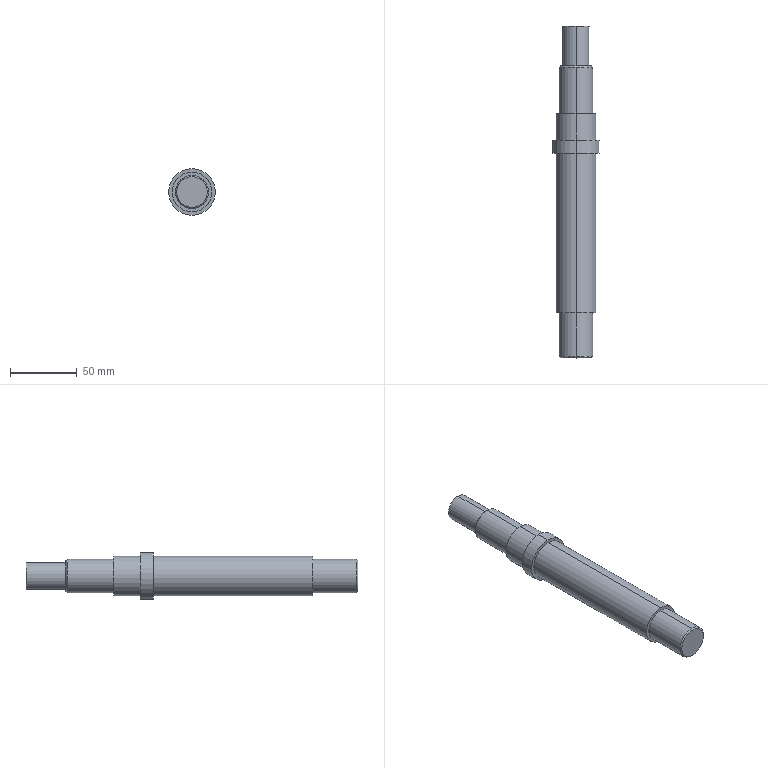Part | STEP file | 012-6-07-05 | 1 solid | 23 faces | box 35 x 249.4 x 35 mm | volume 151867 mm3 | cylinder 12 | plane 7 | cone 4 | commonest cylinder face diameters 25 x4 30 x4 20 x2 35 x2
STEP:
#1=CARTESIAN_POINT('',(0.,0.,0.));
#2=DIRECTION('',(0.,0.,1.));
#3=DIRECTION('',(1.,0.,0.));
#4=AXIS2_PLACEMENT_3D('',#1,#2,#3);
#5=CARTESIAN_POINT('',(0.,219.4,11.5));
#6=VERTEX_POINT('',#5);
#7=CARTESIAN_POINT('',(0.,219.4,-11.5));
#8=VERTEX_POINT('',#7);
#9=CARTESIAN_POINT('',(0.,219.4,0.));
#10=DIRECTION('',(0.,1.,0.));
#11=DIRECTION('',(0.,0.,1.));
#12=AXIS2_PLACEMENT_3D('',#9,#10,#11);
#13=CIRCLE('',#12,11.5);
#14=CARTESIAN_POINT('',(0.,218.4,0.));
#15=DIRECTION('',(0.,-1.,0.));
#16=DIRECTION('',(0.,0.,-1.));
#17=AXIS2_PLACEMENT_3D('',#14,#15,#16);
#18=CONICAL_SURFACE('',#17,12.5,0.7854);
#19=CARTESIAN_POINT('',(3.142,-1.));
#20=DIRECTION('',(-1.,0.));
#21=VECTOR('',#20,1.);
#22=LINE('',#19,#21);
#23=(GEOMETRIC_REPRESENTATION_CONTEXT(2)PARAMETRIC_REPRESENTATION_CONTEXT()REPRESENTATION_CONTEXT('',''));
#24=DEFINITIONAL_REPRESENTATION('',(#22),#23);
#25=PCURVE('',#18,#24);
#26=CARTESIAN_POINT('',(12.5,219.4,0.));
#27=DIRECTION('',(0.,1.,0.));
#28=DIRECTION('',(0.,0.,1.));
#29=AXIS2_PLACEMENT_3D('',#26,#27,#28);
#30=PLANE('',#29);
#31=CARTESIAN_POINT('',(0.,-12.5));
#32=DIRECTION('',(1.,0.));
#33=AXIS2_PLACEMENT_2D('',#31,#32);
#34=CIRCLE('',#33,11.5);
#35=(GEOMETRIC_REPRESENTATION_CONTEXT(2)PARAMETRIC_REPRESENTATION_CONTEXT()REPRESENTATION_CONTEXT('',''));
#36=DEFINITIONAL_REPRESENTATION('',(#34),#35);
#37=PCURVE('',#30,#36);
#38=SURFACE_CURVE('',#13,(#25,#37),.PCURVE_S1.);
#39=EDGE_CURVE('',#6,#8,#38,.T.);
#40=ORIENTED_EDGE('',*,*,#39,.F.);
#41=CARTESIAN_POINT('',(0.,218.4,12.5));
#42=VERTEX_POINT('',#41);
#43=CARTESIAN_POINT('',(0.,218.4,12.5));
#44=DIRECTION('',(0.,-0.7071,0.7071));
#45=VECTOR('',#44,1.);
#46=LINE('',#43,#45);
#47=CARTESIAN_POINT('',(3.142,0.));
#48=DIRECTION('',(0.,1.));
#49=VECTOR('',#48,1.);
#50=LINE('',#47,#49);
#51=(GEOMETRIC_REPRESENTATION_CONTEXT(2)PARAMETRIC_REPRESENTATION_CONTEXT()REPRESENTATION_CONTEXT('',''));
#52=DEFINITIONAL_REPRESENTATION('',(#50),#51);
#53=PCURVE('',#18,#52);
#54=CARTESIAN_POINT('',(0.,218.4,0.));
#55=DIRECTION('',(0.,-1.,0.));
#56=DIRECTION('',(0.,0.,-1.));
#57=AXIS2_PLACEMENT_3D('',#54,#55,#56);
#58=CONICAL_SURFACE('',#57,12.5,0.7854);
#59=CARTESIAN_POINT('',(3.142,0.));
#60=DIRECTION('',(0.,1.));
#61=VECTOR('',#60,1.);
#62=LINE('',#59,#61);
#63=(GEOMETRIC_REPRESENTATION_CONTEXT(2)PARAMETRIC_REPRESENTATION_CONTEXT()REPRESENTATION_CONTEXT('',''));
#64=DEFINITIONAL_REPRESENTATION('',(#62),#63);
#65=PCURVE('',#58,#64);
#66=SURFACE_CURVE('',#46,(#53,#65),.PCURVE_S1.);
#67=EDGE_CURVE('',#6,#42,#66,.T.);
#68=ORIENTED_EDGE('',*,*,#67,.T.);
#69=CARTESIAN_POINT('',(0.,218.4,-12.5));
#70=VERTEX_POINT('',#69);
#71=CARTESIAN_POINT('',(0.,218.4,0.));
#72=DIRECTION('',(0.,-1.,0.));
#73=DIRECTION('',(0.,0.,1.));
#74=AXIS2_PLACEMENT_3D('',#71,#72,#73);
#75=CIRCLE('',#74,12.5);
#76=CARTESIAN_POINT('',(-3.142,0.));
#77=DIRECTION('',(1.,0.));
#78=VECTOR('',#77,1.);
#79=LINE('',#76,#78);
#80=(GEOMETRIC_REPRESENTATION_CONTEXT(2)PARAMETRIC_REPRESENTATION_CONTEXT()REPRESENTATION_CONTEXT('',''));
#81=DEFINITIONAL_REPRESENTATION('',(#79),#80);
#82=PCURVE('',#18,#81);
#83=CARTESIAN_POINT('',(0.,0.,0.));
#84=DIRECTION('',(0.,-1.,0.));
#85=DIRECTION('',(0.,0.,-1.));
#86=AXIS2_PLACEMENT_3D('',#83,#84,#85);
#87=CYLINDRICAL_SURFACE('',#86,12.5);
#88=CARTESIAN_POINT('',(-3.142,-218.4));
#89=DIRECTION('',(1.,0.));
#90=VECTOR('',#89,1.);
#91=LINE('',#88,#90);
#92=(GEOMETRIC_REPRESENTATION_CONTEXT(2)PARAMETRIC_REPRESENTATION_CONTEXT()REPRESENTATION_CONTEXT('',''));
#93=DEFINITIONAL_REPRESENTATION('',(#91),#92);
#94=PCURVE('',#87,#93);
#95=SURFACE_CURVE('',#75,(#82,#94),.PCURVE_S1.);
#96=EDGE_CURVE('',#70,#42,#95,.T.);
#97=ORIENTED_EDGE('',*,*,#96,.F.);
#98=CARTESIAN_POINT('',(0.,218.4,-12.5));
#99=DIRECTION('',(0.,-0.7071,-0.7071));
#100=VECTOR('',#99,1.);
#101=LINE('',#98,#100);
#102=CARTESIAN_POINT('',(0.,0.));
#103=DIRECTION('',(0.,1.));
#104=VECTOR('',#103,1.);
#105=LINE('',#102,#104);
#106=(GEOMETRIC_REPRESENTATION_CONTEXT(2)PARAMETRIC_REPRESENTATION_CONTEXT()REPRESENTATION_CONTEXT('',''));
#107=DEFINITIONAL_REPRESENTATION('',(#105),#106);
#108=PCURVE('',#18,#107);
#109=CARTESIAN_POINT('',(6.283,0.));
#110=DIRECTION('',(0.,1.));
#111=VECTOR('',#110,1.);
#112=LINE('',#109,#111);
#113=(GEOMETRIC_REPRESENTATION_CONTEXT(2)PARAMETRIC_REPRESENTATION_CONTEXT()REPRESENTATION_CONTEXT('',''));
#114=DEFINITIONAL_REPRESENTATION('',(#112),#113);
#115=PCURVE('',#58,#114);
#116=SURFACE_CURVE('',#101,(#108,#115),.PCURVE_S1.);
#117=EDGE_CURVE('',#8,#70,#116,.T.);
#118=ORIENTED_EDGE('',*,*,#117,.F.);
#119=EDGE_LOOP('',(#40,#68,#97,#118));
#120=FACE_BOUND('',#119,.T.);
#121=ADVANCED_FACE('',(#120),#18,.T.);
#122=CARTESIAN_POINT('',(0.,0.,-11.5));
#123=VERTEX_POINT('',#122);
#124=CARTESIAN_POINT('',(0.,0.,11.5));
#125=VERTEX_POINT('',#124);
#126=CARTESIAN_POINT('',(0.,0.,0.));
#127=DIRECTION('',(0.,-1.,0.));
#128=DIRECTION('',(0.,0.,-1.));
#129=AXIS2_PLACEMENT_3D('',#126,#127,#128);
#130=CIRCLE('',#129,11.5);
#131=CARTESIAN_POINT('',(0.,0.,0.));
#132=DIRECTION('',(0.,1.,0.));
#133=DIRECTION('',(0.,0.,1.));
#134=AXIS2_PLACEMENT_3D('',#131,#132,#133);
#135=CONICAL_SURFACE('',#134,11.5,0.7854);
#136=CARTESIAN_POINT('',(3.142,0.));
#137=DIRECTION('',(-1.,0.));
#138=VECTOR('',#137,1.);
#139=LINE('',#136,#138);
#140=(GEOMETRIC_REPRESENTATION_CONTEXT(2)PARAMETRIC_REPRESENTATION_CONTEXT()REPRESENTATION_CONTEXT('',''));
#141=DEFINITIONAL_REPRESENTATION('',(#139),#140);
#142=PCURVE('',#135,#141);
#143=CARTESIAN_POINT('',(0.,0.,0.));
#144=DIRECTION('',(0.,-1.,0.));
#145=DIRECTION('',(0.,0.,-1.));
#146=AXIS2_PLACEMENT_3D('',#143,#144,#145);
#147=PLANE('',#146);
#148=CARTESIAN_POINT('',(0.,0.));
#149=DIRECTION('',(1.,0.));
#150=AXIS2_PLACEMENT_2D('',#148,#149);
#151=CIRCLE('',#150,11.5);
#152=(GEOMETRIC_REPRESENTATION_CONTEXT(2)PARAMETRIC_REPRESENTATION_CONTEXT()REPRESENTATION_CONTEXT('',''));
#153=DEFINITIONAL_REPRESENTATION('',(#151),#152);
#154=PCURVE('',#147,#153);
#155=SURFACE_CURVE('',#130,(#142,#154),.PCURVE_S1.);
#156=EDGE_CURVE('',#123,#125,#155,.T.);
#157=ORIENTED_EDGE('',*,*,#156,.F.);
#158=CARTESIAN_POINT('',(0.,1.,-12.5));
#159=VERTEX_POINT('',#158);
#160=CARTESIAN_POINT('',(0.,0.,-11.5));
#161=DIRECTION('',(0.,0.7071,-0.7071));
#162=VECTOR('',#161,1.);
#163=LINE('',#160,#162);
#164=CARTESIAN_POINT('',(3.142,0.));
#165=DIRECTION('',(0.,1.));
#166=VECTOR('',#165,1.);
#167=LINE('',#164,#166);
#168=(GEOMETRIC_REPRESENTATION_CONTEXT(2)PARAMETRIC_REPRESENTATION_CONTEXT()REPRESENTATION_CONTEXT('',''));
#169=DEFINITIONAL_REPRESENTATION('',(#167),#168);
#170=PCURVE('',#135,#169);
#171=CARTESIAN_POINT('',(0.,0.,0.));
#172=DIRECTION('',(0.,1.,0.));
#173=DIRECTION('',(0.,0.,1.));
#174=AXIS2_PLACEMENT_3D('',#171,#172,#173);
#175=CONICAL_SURFACE('',#174,11.5,0.7854);
#176=CARTESIAN_POINT('',(3.142,0.));
#177=DIRECTION('',(0.,1.));
#178=VECTOR('',#177,1.);
#179=LINE('',#176,#178);
#180=(GEOMETRIC_REPRESENTATION_CONTEXT(2)PARAMETRIC_REPRESENTATION_CONTEXT()REPRESENTATION_CONTEXT('',''));
#181=DEFINITIONAL_REPRESENTATION('',(#179),#180);
#182=PCURVE('',#175,#181);
#183=SURFACE_CURVE('',#163,(#170,#182),.PCURVE_S1.);
#184=EDGE_CURVE('',#123,#159,#183,.T.);
#185=ORIENTED_EDGE('',*,*,#184,.T.);
#186=CARTESIAN_POINT('',(0.,1.,12.5));
#187=VERTEX_POINT('',#186);
#188=CARTESIAN_POINT('',(0.,1.,0.));
#189=DIRECTION('',(0.,1.,0.));
#190=DIRECTION('',(0.,0.,-1.));
#191=AXIS2_PLACEMENT_3D('',#188,#189,#190);
#192=CIRCLE('',#191,12.5);
#193=CARTESIAN_POINT('',(-3.142,1.));
#194=DIRECTION('',(1.,0.));
#195=VECTOR('',#194,1.);
#196=LINE('',#193,#195);
#197=(GEOMETRIC_REPRESENTATION_CONTEXT(2)PARAMETRIC_REPRESENTATION_CONTEXT()REPRESENTATION_CONTEXT('',''));
#198=DEFINITIONAL_REPRESENTATION('',(#196),#197);
#199=PCURVE('',#135,#198);
#200=CARTESIAN_POINT('',(0.,0.,0.));
#201=DIRECTION('',(0.,-1.,0.));
#202=DIRECTION('',(0.,0.,-1.));
#203=AXIS2_PLACEMENT_3D('',#200,#201,#202);
#204=CYLINDRICAL_SURFACE('',#203,12.5);
#205=CARTESIAN_POINT('',(6.283,-1.));
#206=DIRECTION('',(-1.,0.));
#207=VECTOR('',#206,1.);
#208=LINE('',#205,#207);
#209=(GEOMETRIC_REPRESENTATION_CONTEXT(2)PARAMETRIC_REPRESENTATION_CONTEXT()REPRESENTATION_CONTEXT('',''));
#210=DEFINITIONAL_REPRESENTATION('',(#208),#209);
#211=PCURVE('',#204,#210);
#212=SURFACE_CURVE('',#192,(#199,#211),.PCURVE_S1.);
#213=EDGE_CURVE('',#187,#159,#212,.T.);
#214=ORIENTED_EDGE('',*,*,#213,.F.);
#215=CARTESIAN_POINT('',(0.,0.,11.5));
#216=DIRECTION('',(0.,0.7071,0.7071));
#217=VECTOR('',#216,1.);
#218=LINE('',#215,#217);
#219=CARTESIAN_POINT('',(0.,0.));
#220=DIRECTION('',(0.,1.));
#221=VECTOR('',#220,1.);
#222=LINE('',#219,#221);
#223=(GEOMETRIC_REPRESENTATION_CONTEXT(2)PARAMETRIC_REPRESENTATION_CONTEXT()REPRESENTATION_CONTEXT('',''));
#224=DEFINITIONAL_REPRESENTATION('',(#222),#223);
#225=PCURVE('',#135,#224);
#226=CARTESIAN_POINT('',(6.283,0.));
#227=DIRECTION('',(0.,1.));
#228=VECTOR('',#227,1.);
#229=LINE('',#226,#228);
#230=(GEOMETRIC_REPRESENTATION_CONTEXT(2)PARAMETRIC_REPRESENTATION_CONTEXT()REPRESENTATION_CONTEXT('',''));
#231=DEFINITIONAL_REPRESENTATION('',(#229),#230);
#232=PCURVE('',#175,#231);
#233=SURFACE_CURVE('',#218,(#225,#232),.PCURVE_S1.);
#234=EDGE_CURVE('',#125,#187,#233,.T.);
#235=ORIENTED_EDGE('',*,*,#234,.F.);
#236=EDGE_LOOP('',(#157,#185,#214,#235));
#237=FACE_BOUND('',#236,.T.);
#238=ADVANCED_FACE('',(#237),#135,.T.);
#239=CARTESIAN_POINT('',(0.,249.4,-10.));
#240=VERTEX_POINT('',#239);
#241=CARTESIAN_POINT('',(0.,249.4,10.));
#242=VERTEX_POINT('',#241);
#243=CARTESIAN_POINT('',(0.,249.4,0.));
#244=DIRECTION('',(0.,-1.,0.));
#245=DIRECTION('',(0.,0.,-1.));
#246=AXIS2_PLACEMENT_3D('',#243,#244,#245);
#247=CIRCLE('',#246,10.);
#248=CARTESIAN_POINT('',(0.,0.,0.));
#249=DIRECTION('',(0.,-1.,0.));
#250=DIRECTION('',(0.,0.,-1.));
#251=AXIS2_PLACEMENT_3D('',#248,#249,#250);
#252=CYLINDRICAL_SURFACE('',#251,10.);
#253=CARTESIAN_POINT('',(0.,-249.4));
#254=DIRECTION('',(1.,0.));
#255=VECTOR('',#254,1.);
#256=LINE('',#253,#255);
#257=(GEOMETRIC_REPRESENTATION_CONTEXT(2)PARAMETRIC_REPRESENTATION_CONTEXT()REPRESENTATION_CONTEXT('',''));
#258=DEFINITIONAL_REPRESENTATION('',(#256),#257);
#259=PCURVE('',#252,#258);
#260=CARTESIAN_POINT('',(0.,249.4,0.));
#261=DIRECTION('',(0.,1.,0.));
#262=DIRECTION('',(0.,0.,1.));
#263=AXIS2_PLACEMENT_3D('',#260,#261,#262);
#264=PLANE('',#263);
#265=CARTESIAN_POINT('',(-10.,0.));
#266=CARTESIAN_POINT('',(-10.,17.321));
#267=CARTESIAN_POINT('',(5.,8.66));
#268=CARTESIAN_POINT('',(20.,0.));
#269=CARTESIAN_POINT('',(5.,-8.66));
#270=CARTESIAN_POINT('',(-10.,-17.321));
#271=CARTESIAN_POINT('',(-10.,0.));
#272=(BOUNDED_CURVE()B_SPLINE_CURVE(2,(#265,#266,#267,#268,#269,#270,#271),.UNSPECIFIED.,.T.,.F.)B_SPLINE_CURVE_WITH_KNOTS((1,2,2,2,2,1),(-2.094,0.,2.094,4.189,6.283,8.378),.UNSPECIFIED.)CURVE()GEOMETRIC_REPRESENTATION_ITEM()RATIONAL_B_SPLINE_CURVE((1.,0.5,1.,0.5,1.,0.5,1.))REPRESENTATION_ITEM(''));
#273=(GEOMETRIC_REPRESENTATION_CONTEXT(2)PARAMETRIC_REPRESENTATION_CONTEXT()REPRESENTATION_CONTEXT('',''));
#274=DEFINITIONAL_REPRESENTATION('',(#272),#273);
#275=PCURVE('',#264,#274);
#276=SURFACE_CURVE('',#247,(#259,#275),.PCURVE_S1.);
#277=EDGE_CURVE('',#240,#242,#276,.T.);
#278=ORIENTED_EDGE('',*,*,#277,.T.);
#279=CARTESIAN_POINT('',(0.,219.4,10.));
#280=VERTEX_POINT('',#279);
#281=CARTESIAN_POINT('',(0.,0.,10.));
#282=DIRECTION('',(0.,-1.,0.));
#283=VECTOR('',#282,1.);
#284=LINE('',#281,#283);
#285=CARTESIAN_POINT('',(3.142,0.));
#286=DIRECTION('',(0.,1.));
#287=VECTOR('',#286,1.);
#288=LINE('',#285,#287);
#289=(GEOMETRIC_REPRESENTATION_CONTEXT(2)PARAMETRIC_REPRESENTATION_CONTEXT()REPRESENTATION_CONTEXT('',''));
#290=DEFINITIONAL_REPRESENTATION('',(#288),#289);
#291=PCURVE('',#252,#290);
#292=CARTESIAN_POINT('',(0.,0.,0.));
#293=DIRECTION('',(0.,-1.,0.));
#294=DIRECTION('',(0.,0.,-1.));
#295=AXIS2_PLACEMENT_3D('',#292,#293,#294);
#296=CYLINDRICAL_SURFACE('',#295,10.);
#297=CARTESIAN_POINT('',(3.142,0.));
#298=DIRECTION('',(0.,1.));
#299=VECTOR('',#298,1.);
#300=LINE('',#297,#299);
#301=(GEOMETRIC_REPRESENTATION_CONTEXT(2)PARAMETRIC_REPRESENTATION_CONTEXT()REPRESENTATION_CONTEXT('',''));
#302=DEFINITIONAL_REPRESENTATION('',(#300),#301);
#303=PCURVE('',#296,#302);
#304=SURFACE_CURVE('',#284,(#291,#303),.PCURVE_S1.);
#305=EDGE_CURVE('',#242,#280,#304,.T.);
#306=ORIENTED_EDGE('',*,*,#305,.T.);
#307=CARTESIAN_POINT('',(0.,219.4,-10.));
#308=VERTEX_POINT('',#307);
#309=CARTESIAN_POINT('',(0.,219.4,0.));
#310=DIRECTION('',(0.,-1.,0.));
#311=DIRECTION('',(0.,0.,-1.));
#312=AXIS2_PLACEMENT_3D('',#309,#310,#311);
#313=CIRCLE('',#312,10.);
#314=CARTESIAN_POINT('',(0.,-219.4));
#315=DIRECTION('',(1.,0.));
#316=VECTOR('',#315,1.);
#317=LINE('',#314,#316);
#318=(GEOMETRIC_REPRESENTATION_CONTEXT(2)PARAMETRIC_REPRESENTATION_CONTEXT()REPRESENTATION_CONTEXT('',''));
#319=DEFINITIONAL_REPRESENTATION('',(#317),#318);
#320=PCURVE('',#252,#319);
#321=CARTESIAN_POINT('',(-10.,-12.5));
#322=CARTESIAN_POINT('',(-10.,4.821));
#323=CARTESIAN_POINT('',(5.,-3.84));
#324=CARTESIAN_POINT('',(20.,-12.5));
#325=CARTESIAN_POINT('',(5.,-21.16));
#326=CARTESIAN_POINT('',(-10.,-29.821));
#327=CARTESIAN_POINT('',(-10.,-12.5));
#328=(BOUNDED_CURVE()B_SPLINE_CURVE(2,(#321,#322,#323,#324,#325,#326,#327),.UNSPECIFIED.,.T.,.F.)B_SPLINE_CURVE_WITH_KNOTS((1,2,2,2,2,1),(-2.094,0.,2.094,4.189,6.283,8.378),.UNSPECIFIED.)CURVE()GEOMETRIC_REPRESENTATION_ITEM()RATIONAL_B_SPLINE_CURVE((1.,0.5,1.,0.5,1.,0.5,1.))REPRESENTATION_ITEM(''));
#329=(GEOMETRIC_REPRESENTATION_CONTEXT(2)PARAMETRIC_REPRESENTATION_CONTEXT()REPRESENTATION_CONTEXT('',''));
#330=DEFINITIONAL_REPRESENTATION('',(#328),#329);
#331=PCURVE('',#30,#330);
#332=SURFACE_CURVE('',#313,(#320,#331),.PCURVE_S1.);
#333=EDGE_CURVE('',#308,#280,#332,.T.);
#334=ORIENTED_EDGE('',*,*,#333,.F.);
#335=CARTESIAN_POINT('',(0.,0.,-10.));
#336=DIRECTION('',(0.,-1.,0.));
#337=VECTOR('',#336,1.);
#338=LINE('',#335,#337);
#339=CARTESIAN_POINT('',(0.,0.));
#340=DIRECTION('',(0.,1.));
#341=VECTOR('',#340,1.);
#342=LINE('',#339,#341);
#343=(GEOMETRIC_REPRESENTATION_CONTEXT(2)PARAMETRIC_REPRESENTATION_CONTEXT()REPRESENTATION_CONTEXT('',''));
#344=DEFINITIONAL_REPRESENTATION('',(#342),#343);
#345=PCURVE('',#252,#344);
#346=CARTESIAN_POINT('',(6.283,0.));
#347=DIRECTION('',(0.,1.));
#348=VECTOR('',#347,1.);
#349=LINE('',#346,#348);
#350=(GEOMETRIC_REPRESENTATION_CONTEXT(2)PARAMETRIC_REPRESENTATION_CONTEXT()REPRESENTATION_CONTEXT('',''));
#351=DEFINITIONAL_REPRESENTATION('',(#349),#350);
#352=PCURVE('',#296,#351);
#353=SURFACE_CURVE('',#338,(#345,#352),.PCURVE_S1.);
#354=EDGE_CURVE('',#240,#308,#353,.T.);
#355=ORIENTED_EDGE('',*,*,#354,.F.);
#356=EDGE_LOOP('',(#278,#306,#334,#355));
#357=FACE_BOUND('',#356,.T.);
#358=ADVANCED_FACE('',(#357),#252,.T.);
#359=ORIENTED_EDGE('',*,*,#96,.T.);
#360=CARTESIAN_POINT('',(0.,183.4,12.5));
#361=VERTEX_POINT('',#360);
#362=CARTESIAN_POINT('',(0.,0.,12.5));
#363=DIRECTION('',(0.,-1.,0.));
#364=VECTOR('',#363,1.);
#365=LINE('',#362,#364);
#366=CARTESIAN_POINT('',(3.142,0.));
#367=DIRECTION('',(0.,1.));
#368=VECTOR('',#367,1.);
#369=LINE('',#366,#368);
#370=(GEOMETRIC_REPRESENTATION_CONTEXT(2)PARAMETRIC_REPRESENTATION_CONTEXT()REPRESENTATION_CONTEXT('',''));
#371=DEFINITIONAL_REPRESENTATION('',(#369),#370);
#372=PCURVE('',#87,#371);
#373=CARTESIAN_POINT('',(0.,0.,0.));
#374=DIRECTION('',(0.,-1.,0.));
#375=DIRECTION('',(0.,0.,-1.));
#376=AXIS2_PLACEMENT_3D('',#373,#374,#375);
#377=CYLINDRICAL_SURFACE('',#376,12.5);
#378=CARTESIAN_POINT('',(3.142,0.));
#379=DIRECTION('',(0.,1.));
#380=VECTOR('',#379,1.);
#381=LINE('',#378,#380);
#382=(GEOMETRIC_REPRESENTATION_CONTEXT(2)PARAMETRIC_REPRESENTATION_CONTEXT()REPRESENTATION_CONTEXT('',''));
#383=DEFINITIONAL_REPRESENTATION('',(#381),#382);
#384=PCURVE('',#377,#383);
#385=SURFACE_CURVE('',#365,(#372,#384),.PCURVE_S1.);
#386=EDGE_CURVE('',#42,#361,#385,.T.);
#387=ORIENTED_EDGE('',*,*,#386,.T.);
#388=CARTESIAN_POINT('',(0.,183.4,-12.5));
#389=VERTEX_POINT('',#388);
#390=CARTESIAN_POINT('',(0.,183.4,0.));
#391=DIRECTION('',(0.,-1.,0.));
#392=DIRECTION('',(0.,0.,-1.));
#393=AXIS2_PLACEMENT_3D('',#390,#391,#392);
#394=CIRCLE('',#393,12.5);
#395=CARTESIAN_POINT('',(0.,-183.4));
#396=DIRECTION('',(1.,0.));
#397=VECTOR('',#396,1.);
#398=LINE('',#395,#397);
#399=(GEOMETRIC_REPRESENTATION_CONTEXT(2)PARAMETRIC_REPRESENTATION_CONTEXT()REPRESENTATION_CONTEXT('',''));
#400=DEFINITIONAL_REPRESENTATION('',(#398),#399);
#401=PCURVE('',#87,#400);
#402=CARTESIAN_POINT('',(12.5,183.4,0.));
#403=DIRECTION('',(0.,1.,0.));
#404=DIRECTION('',(0.,0.,1.));
#405=AXIS2_PLACEMENT_3D('',#402,#403,#404);
#406=PLANE('',#405);
#407=CARTESIAN_POINT('',(-12.5,-12.5));
#408=CARTESIAN_POINT('',(-12.5,9.151));
#409=CARTESIAN_POINT('',(6.25,-1.675));
#410=CARTESIAN_POINT('',(25.,-12.5));
#411=CARTESIAN_POINT('',(6.25,-23.325));
#412=CARTESIAN_POINT('',(-12.5,-34.151));
#413=CARTESIAN_POINT('',(-12.5,-12.5));
#414=(BOUNDED_CURVE()B_SPLINE_CURVE(2,(#407,#408,#409,#410,#411,#412,#413),.UNSPECIFIED.,.T.,.F.)B_SPLINE_CURVE_WITH_KNOTS((1,2,2,2,2,1),(-2.094,0.,2.094,4.189,6.283,8.378),.UNSPECIFIED.)CURVE()GEOMETRIC_REPRESENTATION_ITEM()RATIONAL_B_SPLINE_CURVE((1.,0.5,1.,0.5,1.,0.5,1.))REPRESENTATION_ITEM(''));
#415=(GEOMETRIC_REPRESENTATION_CONTEXT(2)PARAMETRIC_REPRESENTATION_CONTEXT()REPRESENTATION_CONTEXT('',''));
#416=DEFINITIONAL_REPRESENTATION('',(#414),#415);
#417=PCURVE('',#406,#416);
#418=SURFACE_CURVE('',#394,(#401,#417),.PCURVE_S1.);
#419=EDGE_CURVE('',#389,#361,#418,.T.);
#420=ORIENTED_EDGE('',*,*,#419,.F.);
#421=CARTESIAN_POINT('',(0.,0.,-12.5));
#422=DIRECTION('',(0.,-1.,0.));
#423=VECTOR('',#422,1.);
#424=LINE('',#421,#423);
#425=CARTESIAN_POINT('',(0.,0.));
#426=DIRECTION('',(0.,1.));
#427=VECTOR('',#426,1.);
#428=LINE('',#425,#427);
#429=(GEOMETRIC_REPRESENTATION_CONTEXT(2)PARAMETRIC_REPRESENTATION_CONTEXT()REPRESENTATION_CONTEXT('',''));
#430=DEFINITIONAL_REPRESENTATION('',(#428),#429);
#431=PCURVE('',#87,#430);
#432=CARTESIAN_POINT('',(6.283,0.));
#433=DIRECTION('',(0.,1.));
#434=VECTOR('',#433,1.);
#435=LINE('',#432,#434);
#436=(GEOMETRIC_REPRESENTATION_CONTEXT(2)PARAMETRIC_REPRESENTATION_CONTEXT()REPRESENTATION_CONTEXT('',''));
#437=DEFINITIONAL_REPRESENTATION('',(#435),#436);
#438=PCURVE('',#377,#437);
#439=SURFACE_CURVE('',#424,(#431,#438),.PCURVE_S1.);
#440=EDGE_CURVE('',#70,#389,#439,.T.);
#441=ORIENTED_EDGE('',*,*,#440,.F.);
#442=EDGE_LOOP('',(#359,#387,#420,#441));
#443=FACE_BOUND('',#442,.T.);
#444=ADVANCED_FACE('',(#443),#87,.T.);
#445=CARTESIAN_POINT('',(0.,183.4,-15.));
#446=VERTEX_POINT('',#445);
#447=CARTESIAN_POINT('',(0.,183.4,15.));
#448=VERTEX_POINT('',#447);
#449=CARTESIAN_POINT('',(0.,183.4,0.));
#450=DIRECTION('',(0.,-1.,0.));
#451=DIRECTION('',(0.,0.,-1.));
#452=AXIS2_PLACEMENT_3D('',#449,#450,#451);
#453=CIRCLE('',#452,15.);
#454=CARTESIAN_POINT('',(0.,0.,0.));
#455=DIRECTION('',(0.,-1.,0.));
#456=DIRECTION('',(0.,0.,-1.));
#457=AXIS2_PLACEMENT_3D('',#454,#455,#456);
#458=CYLINDRICAL_SURFACE('',#457,15.);
#459=CARTESIAN_POINT('',(0.,-183.4));
#460=DIRECTION('',(1.,0.));
#461=VECTOR('',#460,1.);
#462=LINE('',#459,#461);
#463=(GEOMETRIC_REPRESENTATION_CONTEXT(2)PARAMETRIC_REPRESENTATION_CONTEXT()REPRESENTATION_CONTEXT('',''));
#464=DEFINITIONAL_REPRESENTATION('',(#462),#463);
#465=PCURVE('',#458,#464);
#466=CARTESIAN_POINT('',(-15.,-12.5));
#467=CARTESIAN_POINT('',(-15.,13.481));
#468=CARTESIAN_POINT('',(7.5,0.4904));
#469=CARTESIAN_POINT('',(30.,-12.5));
#470=CARTESIAN_POINT('',(7.5,-25.49));
#471=CARTESIAN_POINT('',(-15.,-38.481));
#472=CARTESIAN_POINT('',(-15.,-12.5));
#473=(BOUNDED_CURVE()B_SPLINE_CURVE(2,(#466,#467,#468,#469,#470,#471,#472),.UNSPECIFIED.,.T.,.F.)B_SPLINE_CURVE_WITH_KNOTS((1,2,2,2,2,1),(-2.094,0.,2.094,4.189,6.283,8.378),.UNSPECIFIED.)CURVE()GEOMETRIC_REPRESENTATION_ITEM()RATIONAL_B_SPLINE_CURVE((1.,0.5,1.,0.5,1.,0.5,1.))REPRESENTATION_ITEM(''));
#474=(GEOMETRIC_REPRESENTATION_CONTEXT(2)PARAMETRIC_REPRESENTATION_CONTEXT()REPRESENTATION_CONTEXT('',''));
#475=DEFINITIONAL_REPRESENTATION('',(#473),#474);
#476=PCURVE('',#406,#475);
#477=SURFACE_CURVE('',#453,(#465,#476),.PCURVE_S1.);
#478=EDGE_CURVE('',#446,#448,#477,.T.);
#479=ORIENTED_EDGE('',*,*,#478,.T.);
#480=CARTESIAN_POINT('',(0.,163.7,15.));
#481=VERTEX_POINT('',#480);
#482=CARTESIAN_POINT('',(0.,0.,15.));
#483=DIRECTION('',(0.,-1.,0.));
#484=VECTOR('',#483,1.);
#485=LINE('',#482,#484);
#486=CARTESIAN_POINT('',(3.142,0.));
#487=DIRECTION('',(0.,1.));
#488=VECTOR('',#487,1.);
#489=LINE('',#486,#488);
#490=(GEOMETRIC_REPRESENTATION_CONTEXT(2)PARAMETRIC_REPRESENTATION_CONTEXT()REPRESENTATION_CONTEXT('',''));
#491=DEFINITIONAL_REPRESENTATION('',(#489),#490);
#492=PCURVE('',#458,#491);
#493=CARTESIAN_POINT('',(0.,0.,0.));
#494=DIRECTION('',(0.,-1.,0.));
#495=DIRECTION('',(0.,0.,-1.));
#496=AXIS2_PLACEMENT_3D('',#493,#494,#495);
#497=CYLINDRICAL_SURFACE('',#496,15.);
#498=CARTESIAN_POINT('',(3.142,0.));
#499=DIRECTION('',(0.,1.));
#500=VECTOR('',#499,1.);
#501=LINE('',#498,#500);
#502=(GEOMETRIC_REPRESENTATION_CONTEXT(2)PARAMETRIC_REPRESENTATION_CONTEXT()REPRESENTATION_CONTEXT('',''));
#503=DEFINITIONAL_REPRESENTATION('',(#501),#502);
#504=PCURVE('',#497,#503);
#505=SURFACE_CURVE('',#485,(#492,#504),.PCURVE_S1.);
#506=EDGE_CURVE('',#448,#481,#505,.T.);
#507=ORIENTED_EDGE('',*,*,#506,.T.);
#508=CARTESIAN_POINT('',(0.,163.7,-15.));
#509=VERTEX_POINT('',#508);
#510=CARTESIAN_POINT('',(0.,163.7,0.));
#511=DIRECTION('',(0.,-1.,0.));
#512=DIRECTION('',(0.,0.,-1.));
#513=AXIS2_PLACEMENT_3D('',#510,#511,#512);
#514=CIRCLE('',#513,15.);
#515=CARTESIAN_POINT('',(0.,-163.7));
#516=DIRECTION('',(1.,0.));
#517=VECTOR('',#516,1.);
#518=LINE('',#515,#517);
#519=(GEOMETRIC_REPRESENTATION_CONTEXT(2)PARAMETRIC_REPRESENTATION_CONTEXT()REPRESENTATION_CONTEXT('',''));
#520=DEFINITIONAL_REPRESENTATION('',(#518),#519);
#521=PCURVE('',#458,#520);
#522=CARTESIAN_POINT('',(15.,163.7,0.));
#523=DIRECTION('',(0.,1.,0.));
#524=DIRECTION('',(0.,0.,1.));
#525=AXIS2_PLACEMENT_3D('',#522,#523,#524);
#526=PLANE('',#525);
#527=CARTESIAN_POINT('',(-15.,-15.));
#528=CARTESIAN_POINT('',(-15.,10.981));
#529=CARTESIAN_POINT('',(7.5,-2.01));
#530=CARTESIAN_POINT('',(30.,-15.));
#531=CARTESIAN_POINT('',(7.5,-27.99));
#532=CARTESIAN_POINT('',(-15.,-40.981));
#533=CARTESIAN_POINT('',(-15.,-15.));
#534=(BOUNDED_CURVE()B_SPLINE_CURVE(2,(#527,#528,#529,#530,#531,#532,#533),.UNSPECIFIED.,.T.,.F.)B_SPLINE_CURVE_WITH_KNOTS((1,2,2,2,2,1),(-2.094,0.,2.094,4.189,6.283,8.378),.UNSPECIFIED.)CURVE()GEOMETRIC_REPRESENTATION_ITEM()RATIONAL_B_SPLINE_CURVE((1.,0.5,1.,0.5,1.,0.5,1.))REPRESENTATION_ITEM(''));
#535=(GEOMETRIC_REPRESENTATION_CONTEXT(2)PARAMETRIC_REPRESENTATION_CONTEXT()REPRESENTATION_CONTEXT('',''));
#536=DEFINITIONAL_REPRESENTATION('',(#534),#535);
#537=PCURVE('',#526,#536);
#538=SURFACE_CURVE('',#514,(#521,#537),.PCURVE_S1.);
#539=EDGE_CURVE('',#509,#481,#538,.T.);
#540=ORIENTED_EDGE('',*,*,#539,.F.);
#541=CARTESIAN_POINT('',(0.,0.,-15.));
#542=DIRECTION('',(0.,-1.,0.));
#543=VECTOR('',#542,1.);
#544=LINE('',#541,#543);
#545=CARTESIAN_POINT('',(0.,0.));
#546=DIRECTION('',(0.,1.));
#547=VECTOR('',#546,1.);
#548=LINE('',#545,#547);
#549=(GEOMETRIC_REPRESENTATION_CONTEXT(2)PARAMETRIC_REPRESENTATION_CONTEXT()REPRESENTATION_CONTEXT('',''));
#550=DEFINITIONAL_REPRESENTATION('',(#548),#549);
#551=PCURVE('',#458,#550);
#552=CARTESIAN_POINT('',(6.283,0.));
#553=DIRECTION('',(0.,1.));
#554=VECTOR('',#553,1.);
#555=LINE('',#552,#554);
#556=(GEOMETRIC_REPRESENTATION_CONTEXT(2)PARAMETRIC_REPRESENTATION_CONTEXT()REPRESENTATION_CONTEXT('',''));
#557=DEFINITIONAL_REPRESENTATION('',(#555),#556);
#558=PCURVE('',#497,#557);
#559=SURFACE_CURVE('',#544,(#551,#558),.PCURVE_S1.);
#560=EDGE_CURVE('',#446,#509,#559,.T.);
#561=ORIENTED_EDGE('',*,*,#560,.F.);
#562=EDGE_LOOP('',(#479,#507,#540,#561));
#563=FACE_BOUND('',#562,.T.);
#564=ADVANCED_FACE('',(#563),#458,.T.);
#565=CARTESIAN_POINT('',(0.,163.7,-17.5));
#566=VERTEX_POINT('',#565);
#567=CARTESIAN_POINT('',(0.,163.7,17.5));
#568=VERTEX_POINT('',#567);
#569=CARTESIAN_POINT('',(0.,163.7,0.));
#570=DIRECTION('',(0.,-1.,0.));
#571=DIRECTION('',(0.,0.,-1.));
#572=AXIS2_PLACEMENT_3D('',#569,#570,#571);
#573=CIRCLE('',#572,17.5);
#574=CARTESIAN_POINT('',(0.,0.,0.));
#575=DIRECTION('',(0.,-1.,0.));
#576=DIRECTION('',(0.,0.,-1.));
#577=AXIS2_PLACEMENT_3D('',#574,#575,#576);
#578=CYLINDRICAL_SURFACE('',#577,17.5);
#579=CARTESIAN_POINT('',(0.,-163.7));
#580=DIRECTION('',(1.,0.));
#581=VECTOR('',#580,1.);
#582=LINE('',#579,#581);
#583=(GEOMETRIC_REPRESENTATION_CONTEXT(2)PARAMETRIC_REPRESENTATION_CONTEXT()REPRESENTATION_CONTEXT('',''));
#584=DEFINITIONAL_REPRESENTATION('',(#582),#583);
#585=PCURVE('',#578,#584);
#586=CARTESIAN_POINT('',(-17.5,-15.));
#587=CARTESIAN_POINT('',(-17.5,15.311));
#588=CARTESIAN_POINT('',(8.75,0.1554));
#589=CARTESIAN_POINT('',(35.,-15.));
#590=CARTESIAN_POINT('',(8.75,-30.155));
#591=CARTESIAN_POINT('',(-17.5,-45.311));
#592=CARTESIAN_POINT('',(-17.5,-15.));
#593=(BOUNDED_CURVE()B_SPLINE_CURVE(2,(#586,#587,#588,#589,#590,#591,#592),.UNSPECIFIED.,.T.,.F.)B_SPLINE_CURVE_WITH_KNOTS((1,2,2,2,2,1),(-2.094,0.,2.094,4.189,6.283,8.378),.UNSPECIFIED.)CURVE()GEOMETRIC_REPRESENTATION_ITEM()RATIONAL_B_SPLINE_CURVE((1.,0.5,1.,0.5,1.,0.5,1.))REPRESENTATION_ITEM(''));
#594=(GEOMETRIC_REPRESENTATION_CONTEXT(2)PARAMETRIC_REPRESENTATION_CONTEXT()REPRESENTATION_CONTEXT('',''));
#595=DEFINITIONAL_REPRESENTATION('',(#593),#594);
#596=PCURVE('',#526,#595);
#597=SURFACE_CURVE('',#573,(#585,#596),.PCURVE_S1.);
#598=EDGE_CURVE('',#566,#568,#597,.T.);
#599=ORIENTED_EDGE('',*,*,#598,.T.);
#600=CARTESIAN_POINT('',(0.,153.7,17.5));
#601=VERTEX_POINT('',#600);
#602=CARTESIAN_POINT('',(0.,0.,17.5));
#603=DIRECTION('',(0.,-1.,0.));
#604=VECTOR('',#603,1.);
#605=LINE('',#602,#604);
#606=CARTESIAN_POINT('',(3.142,0.));
#607=DIRECTION('',(0.,1.));
#608=VECTOR('',#607,1.);
#609=LINE('',#606,#608);
#610=(GEOMETRIC_REPRESENTATION_CONTEXT(2)PARAMETRIC_REPRESENTATION_CONTEXT()REPRESENTATION_CONTEXT('',''));
#611=DEFINITIONAL_REPRESENTATION('',(#609),#610);
#612=PCURVE('',#578,#611);
#613=CARTESIAN_POINT('',(0.,0.,0.));
#614=DIRECTION('',(0.,-1.,0.));
#615=DIRECTION('',(0.,0.,-1.));
#616=AXIS2_PLACEMENT_3D('',#613,#614,#615);
#617=CYLINDRICAL_SURFACE('',#616,17.5);
#618=CARTESIAN_POINT('',(3.142,0.));
#619=DIRECTION('',(0.,1.));
#620=VECTOR('',#619,1.);
#621=LINE('',#618,#620);
#622=(GEOMETRIC_REPRESENTATION_CONTEXT(2)PARAMETRIC_REPRESENTATION_CONTEXT()REPRESENTATION_CONTEXT('',''));
#623=DEFINITIONAL_REPRESENTATION('',(#621),#622);
#624=PCURVE('',#617,#623);
#625=SURFACE_CURVE('',#605,(#612,#624),.PCURVE_S1.);
#626=EDGE_CURVE('',#568,#601,#625,.T.);
#627=ORIENTED_EDGE('',*,*,#626,.T.);
#628=CARTESIAN_POINT('',(0.,153.7,-17.5));
#629=VERTEX_POINT('',#628);
#630=CARTESIAN_POINT('',(0.,153.7,0.));
#631=DIRECTION('',(0.,-1.,0.));
#632=DIRECTION('',(0.,0.,-1.));
#633=AXIS2_PLACEMENT_3D('',#630,#631,#632);
#634=CIRCLE('',#633,17.5);
#635=CARTESIAN_POINT('',(0.,-153.7));
#636=DIRECTION('',(1.,0.));
#637=VECTOR('',#636,1.);
#638=LINE('',#635,#637);
#639=(GEOMETRIC_REPRESENTATION_CONTEXT(2)PARAMETRIC_REPRESENTATION_CONTEXT()REPRESENTATION_CONTEXT('',''));
#640=DEFINITIONAL_REPRESENTATION('',(#638),#639);
#641=PCURVE('',#578,#640);
#642=CARTESIAN_POINT('',(17.5,153.7,0.));
#643=DIRECTION('',(0.,-1.,0.));
#644=DIRECTION('',(0.,0.,-1.));
#645=AXIS2_PLACEMENT_3D('',#642,#643,#644);
#646=PLANE('',#645);
#647=CARTESIAN_POINT('',(0.,-17.5));
#648=DIRECTION('',(1.,0.));
#649=AXIS2_PLACEMENT_2D('',#647,#648);
#650=CIRCLE('',#649,17.5);
#651=(GEOMETRIC_REPRESENTATION_CONTEXT(2)PARAMETRIC_REPRESENTATION_CONTEXT()REPRESENTATION_CONTEXT('',''));
#652=DEFINITIONAL_REPRESENTATION('',(#650),#651);
#653=PCURVE('',#646,#652);
#654=SURFACE_CURVE('',#634,(#641,#653),.PCURVE_S1.);
#655=EDGE_CURVE('',#629,#601,#654,.T.);
#656=ORIENTED_EDGE('',*,*,#655,.F.);
#657=CARTESIAN_POINT('',(0.,0.,-17.5));
#658=DIRECTION('',(0.,-1.,0.));
#659=VECTOR('',#658,1.);
#660=LINE('',#657,#659);
#661=CARTESIAN_POINT('',(0.,0.));
#662=DIRECTION('',(0.,1.));
#663=VECTOR('',#662,1.);
#664=LINE('',#661,#663);
#665=(GEOMETRIC_REPRESENTATION_CONTEXT(2)PARAMETRIC_REPRESENTATION_CONTEXT()REPRESENTATION_CONTEXT('',''));
#666=DEFINITIONAL_REPRESENTATION('',(#664),#665);
#667=PCURVE('',#578,#666);
#668=CARTESIAN_POINT('',(6.283,0.));
#669=DIRECTION('',(0.,1.));
#670=VECTOR('',#669,1.);
#671=LINE('',#668,#670);
#672=(GEOMETRIC_REPRESENTATION_CONTEXT(2)PARAMETRIC_REPRESENTATION_CONTEXT()REPRESENTATION_CONTEXT('',''));
#673=DEFINITIONAL_REPRESENTATION('',(#671),#672);
#674=PCURVE('',#617,#673);
#675=SURFACE_CURVE('',#660,(#667,#674),.PCURVE_S1.);
#676=EDGE_CURVE('',#566,#629,#675,.T.);
#677=ORIENTED_EDGE('',*,*,#676,.F.);
#678=EDGE_LOOP('',(#599,#627,#656,#677));
#679=FACE_BOUND('',#678,.T.);
#680=ADVANCED_FACE('',(#679),#578,.T.);
#681=CARTESIAN_POINT('',(0.,153.7,-15.));
#682=VERTEX_POINT('',#681);
#683=CARTESIAN_POINT('',(0.,153.7,15.));
#684=VERTEX_POINT('',#683);
#685=CARTESIAN_POINT('',(0.,153.7,0.));
#686=DIRECTION('',(0.,-1.,0.));
#687=DIRECTION('',(0.,0.,-1.));
#688=AXIS2_PLACEMENT_3D('',#685,#686,#687);
#689=CIRCLE('',#688,15.);
#690=CARTESIAN_POINT('',(0.,0.,0.));
#691=DIRECTION('',(0.,-1.,0.));
#692=DIRECTION('',(0.,0.,-1.));
#693=AXIS2_PLACEMENT_3D('',#690,#691,#692);
#694=CYLINDRICAL_SURFACE('',#693,15.);
#695=CARTESIAN_POINT('',(0.,-153.7));
#696=DIRECTION('',(1.,0.));
#697=VECTOR('',#696,1.);
#698=LINE('',#695,#697);
#699=(GEOMETRIC_REPRESENTATION_CONTEXT(2)PARAMETRIC_REPRESENTATION_CONTEXT()REPRESENTATION_CONTEXT('',''));
#700=DEFINITIONAL_REPRESENTATION('',(#698),#699);
#701=PCURVE('',#694,#700);
#702=CARTESIAN_POINT('',(0.,-17.5));
#703=DIRECTION('',(1.,0.));
#704=AXIS2_PLACEMENT_2D('',#702,#703);
#705=CIRCLE('',#704,15.);
#706=(GEOMETRIC_REPRESENTATION_CONTEXT(2)PARAMETRIC_REPRESENTATION_CONTEXT()REPRESENTATION_CONTEXT('',''));
#707=DEFINITIONAL_REPRESENTATION('',(#705),#706);
#708=PCURVE('',#646,#707);
#709=SURFACE_CURVE('',#689,(#701,#708),.PCURVE_S1.);
#710=EDGE_CURVE('',#682,#684,#709,.T.);
#711=ORIENTED_EDGE('',*,*,#710,.T.);
#712=CARTESIAN_POINT('',(0.,34.,15.));
#713=VERTEX_POINT('',#712);
#714=CARTESIAN_POINT('',(0.,0.,15.));
#715=DIRECTION('',(0.,-1.,0.));
#716=VECTOR('',#715,1.);
#717=LINE('',#714,#716);
#718=CARTESIAN_POINT('',(3.142,0.));
#719=DIRECTION('',(0.,1.));
#720=VECTOR('',#719,1.);
#721=LINE('',#718,#720);
#722=(GEOMETRIC_REPRESENTATION_CONTEXT(2)PARAMETRIC_REPRESENTATION_CONTEXT()REPRESENTATION_CONTEXT('',''));
#723=DEFINITIONAL_REPRESENTATION('',(#721),#722);
#724=PCURVE('',#694,#723);
#725=CARTESIAN_POINT('',(0.,0.,0.));
#726=DIRECTION('',(0.,-1.,0.));
#727=DIRECTION('',(0.,0.,-1.));
#728=AXIS2_PLACEMENT_3D('',#725,#726,#727);
#729=CYLINDRICAL_SURFACE('',#728,15.);
#730=CARTESIAN_POINT('',(3.142,0.));
#731=DIRECTION('',(0.,1.));
#732=VECTOR('',#731,1.);
#733=LINE('',#730,#732);
#734=(GEOMETRIC_REPRESENTATION_CONTEXT(2)PARAMETRIC_REPRESENTATION_CONTEXT()REPRESENTATION_CONTEXT('',''));
#735=DEFINITIONAL_REPRESENTATION('',(#733),#734);
#736=PCURVE('',#729,#735);
#737=SURFACE_CURVE('',#717,(#724,#736),.PCURVE_S1.);
#738=EDGE_CURVE('',#684,#713,#737,.T.);
#739=ORIENTED_EDGE('',*,*,#738,.T.);
#740=CARTESIAN_POINT('',(0.,34.,-15.));
#741=VERTEX_POINT('',#740);
#742=CARTESIAN_POINT('',(0.,34.,0.));
#743=DIRECTION('',(0.,-1.,0.));
#744=DIRECTION('',(0.,0.,-1.));
#745=AXIS2_PLACEMENT_3D('',#742,#743,#744);
#746=CIRCLE('',#745,15.);
#747=CARTESIAN_POINT('',(0.,-34.));
#748=DIRECTION('',(1.,0.));
#749=VECTOR('',#748,1.);
#750=LINE('',#747,#749);
#751=(GEOMETRIC_REPRESENTATION_CONTEXT(2)PARAMETRIC_REPRESENTATION_CONTEXT()REPRESENTATION_CONTEXT('',''));
#752=DEFINITIONAL_REPRESENTATION('',(#750),#751);
#753=PCURVE('',#694,#752);
#754=CARTESIAN_POINT('',(12.5,34.,0.));
#755=DIRECTION('',(0.,-1.,0.));
#756=DIRECTION('',(0.,0.,-1.));
#757=AXIS2_PLACEMENT_3D('',#754,#755,#756);
#758=PLANE('',#757);
#759=CARTESIAN_POINT('',(0.,-12.5));
#760=DIRECTION('',(1.,0.));
#761=AXIS2_PLACEMENT_2D('',#759,#760);
#762=CIRCLE('',#761,15.);
#763=(GEOMETRIC_REPRESENTATION_CONTEXT(2)PARAMETRIC_REPRESENTATION_CONTEXT()REPRESENTATION_CONTEXT('',''));
#764=DEFINITIONAL_REPRESENTATION('',(#762),#763);
#765=PCURVE('',#758,#764);
#766=SURFACE_CURVE('',#746,(#753,#765),.PCURVE_S1.);
#767=EDGE_CURVE('',#741,#713,#766,.T.);
#768=ORIENTED_EDGE('',*,*,#767,.F.);
#769=CARTESIAN_POINT('',(0.,0.,-15.));
#770=DIRECTION('',(0.,-1.,0.));
#771=VECTOR('',#770,1.);
#772=LINE('',#769,#771);
#773=CARTESIAN_POINT('',(0.,0.));
#774=DIRECTION('',(0.,1.));
#775=VECTOR('',#774,1.);
#776=LINE('',#773,#775);
#777=(GEOMETRIC_REPRESENTATION_CONTEXT(2)PARAMETRIC_REPRESENTATION_CONTEXT()REPRESENTATION_CONTEXT('',''));
#778=DEFINITIONAL_REPRESENTATION('',(#776),#777);
#779=PCURVE('',#694,#778);
#780=CARTESIAN_POINT('',(6.283,0.));
#781=DIRECTION('',(0.,1.));
#782=VECTOR('',#781,1.);
#783=LINE('',#780,#782);
#784=(GEOMETRIC_REPRESENTATION_CONTEXT(2)PARAMETRIC_REPRESENTATION_CONTEXT()REPRESENTATION_CONTEXT('',''));
#785=DEFINITIONAL_REPRESENTATION('',(#783),#784);
#786=PCURVE('',#729,#785);
#787=SURFACE_CURVE('',#772,(#779,#786),.PCURVE_S1.);
#788=EDGE_CURVE('',#682,#741,#787,.T.);
#789=ORIENTED_EDGE('',*,*,#788,.F.);
#790=EDGE_LOOP('',(#711,#739,#768,#789));
#791=FACE_BOUND('',#790,.T.);
#792=ADVANCED_FACE('',(#791),#694,.T.);
#793=CARTESIAN_POINT('',(0.,34.,-12.5));
#794=VERTEX_POINT('',#793);
#795=CARTESIAN_POINT('',(0.,34.,12.5));
#796=VERTEX_POINT('',#795);
#797=CARTESIAN_POINT('',(0.,34.,0.));
#798=DIRECTION('',(0.,-1.,0.));
#799=DIRECTION('',(0.,0.,-1.));
#800=AXIS2_PLACEMENT_3D('',#797,#798,#799);
#801=CIRCLE('',#800,12.5);
#802=CARTESIAN_POINT('',(0.,-34.));
#803=DIRECTION('',(1.,0.));
#804=VECTOR('',#803,1.);
#805=LINE('',#802,#804);
#806=(GEOMETRIC_REPRESENTATION_CONTEXT(2)PARAMETRIC_REPRESENTATION_CONTEXT()REPRESENTATION_CONTEXT('',''));
#807=DEFINITIONAL_REPRESENTATION('',(#805),#806);
#808=PCURVE('',#204,#807);
#809=CARTESIAN_POINT('',(0.,-12.5));
#810=DIRECTION('',(1.,0.));
#811=AXIS2_PLACEMENT_2D('',#809,#810);
#812=CIRCLE('',#811,12.5);
#813=(GEOMETRIC_REPRESENTATION_CONTEXT(2)PARAMETRIC_REPRESENTATION_CONTEXT()REPRESENTATION_CONTEXT('',''));
#814=DEFINITIONAL_REPRESENTATION('',(#812),#813);
#815=PCURVE('',#758,#814);
#816=SURFACE_CURVE('',#801,(#808,#815),.PCURVE_S1.);
#817=EDGE_CURVE('',#794,#796,#816,.T.);
#818=ORIENTED_EDGE('',*,*,#817,.T.);
#819=CARTESIAN_POINT('',(0.,0.,12.5));
#820=DIRECTION('',(0.,-1.,0.));
#821=VECTOR('',#820,1.);
#822=LINE('',#819,#821);
#823=CARTESIAN_POINT('',(3.142,0.));
#824=DIRECTION('',(0.,1.));
#825=VECTOR('',#824,1.);
#826=LINE('',#823,#825);
#827=(GEOMETRIC_REPRESENTATION_CONTEXT(2)PARAMETRIC_REPRESENTATION_CONTEXT()REPRESENTATION_CONTEXT('',''));
#828=DEFINITIONAL_REPRESENTATION('',(#826),#827);
#829=PCURVE('',#204,#828);
#830=CARTESIAN_POINT('',(0.,0.,0.));
#831=DIRECTION('',(0.,-1.,0.));
#832=DIRECTION('',(0.,0.,-1.));
#833=AXIS2_PLACEMENT_3D('',#830,#831,#832);
#834=CYLINDRICAL_SURFACE('',#833,12.5);
#835=CARTESIAN_POINT('',(3.142,0.));
#836=DIRECTION('',(0.,1.));
#837=VECTOR('',#836,1.);
#838=LINE('',#835,#837);
#839=(GEOMETRIC_REPRESENTATION_CONTEXT(2)PARAMETRIC_REPRESENTATION_CONTEXT()REPRESENTATION_CONTEXT('',''));
#840=DEFINITIONAL_REPRESENTATION('',(#838),#839);
#841=PCURVE('',#834,#840);
#842=SURFACE_CURVE('',#822,(#829,#841),.PCURVE_S1.);
#843=EDGE_CURVE('',#796,#187,#842,.T.);
#844=ORIENTED_EDGE('',*,*,#843,.T.);
#845=ORIENTED_EDGE('',*,*,#213,.T.);
#846=CARTESIAN_POINT('',(0.,0.,-12.5));
#847=DIRECTION('',(0.,-1.,0.));
#848=VECTOR('',#847,1.);
#849=LINE('',#846,#848);
#850=CARTESIAN_POINT('',(0.,0.));
#851=DIRECTION('',(0.,1.));
#852=VECTOR('',#851,1.);
#853=LINE('',#850,#852);
#854=(GEOMETRIC_REPRESENTATION_CONTEXT(2)PARAMETRIC_REPRESENTATION_CONTEXT()REPRESENTATION_CONTEXT('',''));
#855=DEFINITIONAL_REPRESENTATION('',(#853),#854);
#856=PCURVE('',#204,#855);
#857=CARTESIAN_POINT('',(6.283,0.));
#858=DIRECTION('',(0.,1.));
#859=VECTOR('',#858,1.);
#860=LINE('',#857,#859);
#861=(GEOMETRIC_REPRESENTATION_CONTEXT(2)PARAMETRIC_REPRESENTATION_CONTEXT()REPRESENTATION_CONTEXT('',''));
#862=DEFINITIONAL_REPRESENTATION('',(#860),#861);
#863=PCURVE('',#834,#862);
#864=SURFACE_CURVE('',#849,(#856,#863),.PCURVE_S1.);
#865=EDGE_CURVE('',#794,#159,#864,.T.);
#866=ORIENTED_EDGE('',*,*,#865,.F.);
#867=EDGE_LOOP('',(#818,#844,#845,#866));
#868=FACE_BOUND('',#867,.T.);
#869=ADVANCED_FACE('',(#868),#204,.T.);
#870=CARTESIAN_POINT('',(0.,0.,0.));
#871=DIRECTION('',(0.,-1.,0.));
#872=DIRECTION('',(0.,0.,-1.));
#873=AXIS2_PLACEMENT_3D('',#870,#871,#872);
#874=CIRCLE('',#873,11.5);
#875=CARTESIAN_POINT('',(0.,0.));
#876=DIRECTION('',(1.,0.));
#877=AXIS2_PLACEMENT_2D('',#875,#876);
#878=CIRCLE('',#877,11.5);
#879=(GEOMETRIC_REPRESENTATION_CONTEXT(2)PARAMETRIC_REPRESENTATION_CONTEXT()REPRESENTATION_CONTEXT('',''));
#880=DEFINITIONAL_REPRESENTATION('',(#878),#879);
#881=PCURVE('',#147,#880);
#882=CARTESIAN_POINT('',(9.425,0.));
#883=DIRECTION('',(-1.,0.));
#884=VECTOR('',#883,1.);
#885=LINE('',#882,#884);
#886=(GEOMETRIC_REPRESENTATION_CONTEXT(2)PARAMETRIC_REPRESENTATION_CONTEXT()REPRESENTATION_CONTEXT('',''));
#887=DEFINITIONAL_REPRESENTATION('',(#885),#886);
#888=PCURVE('',#175,#887);
#889=SURFACE_CURVE('',#874,(#881,#888),.PCURVE_S1.);
#890=EDGE_CURVE('',#125,#123,#889,.T.);
#891=ORIENTED_EDGE('',*,*,#890,.T.);
#892=ORIENTED_EDGE('',*,*,#156,.T.);
#893=EDGE_LOOP('',(#891,#892));
#894=FACE_BOUND('',#893,.T.);
#895=ADVANCED_FACE('',(#894),#147,.T.);
#896=ORIENTED_EDGE('',*,*,#843,.F.);
#897=CARTESIAN_POINT('',(0.,34.,0.));
#898=DIRECTION('',(0.,-1.,0.));
#899=DIRECTION('',(0.,0.,-1.));
#900=AXIS2_PLACEMENT_3D('',#897,#898,#899);
#901=CIRCLE('',#900,12.5);
#902=CARTESIAN_POINT('',(0.,-34.));
#903=DIRECTION('',(1.,0.));
#904=VECTOR('',#903,1.);
#905=LINE('',#902,#904);
#906=(GEOMETRIC_REPRESENTATION_CONTEXT(2)PARAMETRIC_REPRESENTATION_CONTEXT()REPRESENTATION_CONTEXT('',''));
#907=DEFINITIONAL_REPRESENTATION('',(#905),#906);
#908=PCURVE('',#834,#907);
#909=CARTESIAN_POINT('',(0.,-12.5));
#910=DIRECTION('',(1.,0.));
#911=AXIS2_PLACEMENT_2D('',#909,#910);
#912=CIRCLE('',#911,12.5);
#913=(GEOMETRIC_REPRESENTATION_CONTEXT(2)PARAMETRIC_REPRESENTATION_CONTEXT()REPRESENTATION_CONTEXT('',''));
#914=DEFINITIONAL_REPRESENTATION('',(#912),#913);
#915=PCURVE('',#758,#914);
#916=SURFACE_CURVE('',#901,(#908,#915),.PCURVE_S1.);
#917=EDGE_CURVE('',#796,#794,#916,.T.);
#918=ORIENTED_EDGE('',*,*,#917,.T.);
#919=ORIENTED_EDGE('',*,*,#865,.T.);
#920=CARTESIAN_POINT('',(0.,1.,0.));
#921=DIRECTION('',(0.,1.,0.));
#922=DIRECTION('',(0.,0.,-1.));
#923=AXIS2_PLACEMENT_3D('',#920,#921,#922);
#924=CIRCLE('',#923,12.5);
#925=CARTESIAN_POINT('',(6.283,-1.));
#926=DIRECTION('',(-1.,0.));
#927=VECTOR('',#926,1.);
#928=LINE('',#925,#927);
#929=(GEOMETRIC_REPRESENTATION_CONTEXT(2)PARAMETRIC_REPRESENTATION_CONTEXT()REPRESENTATION_CONTEXT('',''));
#930=DEFINITIONAL_REPRESENTATION('',(#928),#929);
#931=PCURVE('',#834,#930);
#932=CARTESIAN_POINT('',(3.142,1.));
#933=DIRECTION('',(1.,0.));
#934=VECTOR('',#933,1.);
#935=LINE('',#932,#934);
#936=(GEOMETRIC_REPRESENTATION_CONTEXT(2)PARAMETRIC_REPRESENTATION_CONTEXT()REPRESENTATION_CONTEXT('',''));
#937=DEFINITIONAL_REPRESENTATION('',(#935),#936);
#938=PCURVE('',#175,#937);
#939=SURFACE_CURVE('',#924,(#931,#938),.PCURVE_S1.);
#940=EDGE_CURVE('',#159,#187,#939,.T.);
#941=ORIENTED_EDGE('',*,*,#940,.T.);
#942=EDGE_LOOP('',(#896,#918,#919,#941));
#943=FACE_BOUND('',#942,.T.);
#944=ADVANCED_FACE('',(#943),#834,.T.);
#945=ORIENTED_EDGE('',*,*,#767,.T.);
#946=CARTESIAN_POINT('',(0.,34.,0.));
#947=DIRECTION('',(0.,-1.,0.));
#948=DIRECTION('',(0.,0.,-1.));
#949=AXIS2_PLACEMENT_3D('',#946,#947,#948);
#950=CIRCLE('',#949,15.);
#951=CARTESIAN_POINT('',(0.,-12.5));
#952=DIRECTION('',(1.,0.));
#953=AXIS2_PLACEMENT_2D('',#951,#952);
#954=CIRCLE('',#953,15.);
#955=(GEOMETRIC_REPRESENTATION_CONTEXT(2)PARAMETRIC_REPRESENTATION_CONTEXT()REPRESENTATION_CONTEXT('',''));
#956=DEFINITIONAL_REPRESENTATION('',(#954),#955);
#957=PCURVE('',#758,#956);
#958=CARTESIAN_POINT('',(0.,-34.));
#959=DIRECTION('',(1.,0.));
#960=VECTOR('',#959,1.);
#961=LINE('',#958,#960);
#962=(GEOMETRIC_REPRESENTATION_CONTEXT(2)PARAMETRIC_REPRESENTATION_CONTEXT()REPRESENTATION_CONTEXT('',''));
#963=DEFINITIONAL_REPRESENTATION('',(#961),#962);
#964=PCURVE('',#729,#963);
#965=SURFACE_CURVE('',#950,(#957,#964),.PCURVE_S1.);
#966=EDGE_CURVE('',#713,#741,#965,.T.);
#967=ORIENTED_EDGE('',*,*,#966,.T.);
#968=EDGE_LOOP('',(#945,#967));
#969=FACE_BOUND('',#968,.T.);
#970=ORIENTED_EDGE('',*,*,#817,.F.);
#971=ORIENTED_EDGE('',*,*,#917,.F.);
#972=EDGE_LOOP('',(#970,#971));
#973=FACE_BOUND('',#972,.T.);
#974=ADVANCED_FACE('',(#969,#973),#758,.T.);
#975=ORIENTED_EDGE('',*,*,#738,.F.);
#976=CARTESIAN_POINT('',(0.,153.7,0.));
#977=DIRECTION('',(0.,-1.,0.));
#978=DIRECTION('',(0.,0.,-1.));
#979=AXIS2_PLACEMENT_3D('',#976,#977,#978);
#980=CIRCLE('',#979,15.);
#981=CARTESIAN_POINT('',(0.,-153.7));
#982=DIRECTION('',(1.,0.));
#983=VECTOR('',#982,1.);
#984=LINE('',#981,#983);
#985=(GEOMETRIC_REPRESENTATION_CONTEXT(2)PARAMETRIC_REPRESENTATION_CONTEXT()REPRESENTATION_CONTEXT('',''));
#986=DEFINITIONAL_REPRESENTATION('',(#984),#985);
#987=PCURVE('',#729,#986);
#988=CARTESIAN_POINT('',(0.,-17.5));
#989=DIRECTION('',(1.,0.));
#990=AXIS2_PLACEMENT_2D('',#988,#989);
#991=CIRCLE('',#990,15.);
#992=(GEOMETRIC_REPRESENTATION_CONTEXT(2)PARAMETRIC_REPRESENTATION_CONTEXT()REPRESENTATION_CONTEXT('',''));
#993=DEFINITIONAL_REPRESENTATION('',(#991),#992);
#994=PCURVE('',#646,#993);
#995=SURFACE_CURVE('',#980,(#987,#994),.PCURVE_S1.);
#996=EDGE_CURVE('',#684,#682,#995,.T.);
#997=ORIENTED_EDGE('',*,*,#996,.T.);
#998=ORIENTED_EDGE('',*,*,#788,.T.);
#999=ORIENTED_EDGE('',*,*,#966,.F.);
#1000=EDGE_LOOP('',(#975,#997,#998,#999));
#1001=FACE_BOUND('',#1000,.T.);
#1002=ADVANCED_FACE('',(#1001),#729,.T.);
#1003=ORIENTED_EDGE('',*,*,#655,.T.);
#1004=CARTESIAN_POINT('',(0.,153.7,0.));
#1005=DIRECTION('',(0.,-1.,0.));
#1006=DIRECTION('',(0.,0.,-1.));
#1007=AXIS2_PLACEMENT_3D('',#1004,#1005,#1006);
#1008=CIRCLE('',#1007,17.5);
#1009=CARTESIAN_POINT('',(0.,-17.5));
#1010=DIRECTION('',(1.,0.));
#1011=AXIS2_PLACEMENT_2D('',#1009,#1010);
#1012=CIRCLE('',#1011,17.5);
#1013=(GEOMETRIC_REPRESENTATION_CONTEXT(2)PARAMETRIC_REPRESENTATION_CONTEXT()REPRESENTATION_CONTEXT('',''));
#1014=DEFINITIONAL_REPRESENTATION('',(#1012),#1013);
#1015=PCURVE('',#646,#1014);
#1016=CARTESIAN_POINT('',(0.,-153.7));
#1017=DIRECTION('',(1.,0.));
#1018=VECTOR('',#1017,1.);
#1019=LINE('',#1016,#1018);
#1020=(GEOMETRIC_REPRESENTATION_CONTEXT(2)PARAMETRIC_REPRESENTATION_CONTEXT()REPRESENTATION_CONTEXT('',''));
#1021=DEFINITIONAL_REPRESENTATION('',(#1019),#1020);
#1022=PCURVE('',#617,#1021);
#1023=SURFACE_CURVE('',#1008,(#1015,#1022),.PCURVE_S1.);
#1024=EDGE_CURVE('',#601,#629,#1023,.T.);
#1025=ORIENTED_EDGE('',*,*,#1024,.T.);
#1026=EDGE_LOOP('',(#1003,#1025));
#1027=FACE_BOUND('',#1026,.T.);
#1028=ORIENTED_EDGE('',*,*,#710,.F.);
#1029=ORIENTED_EDGE('',*,*,#996,.F.);
#1030=EDGE_LOOP('',(#1028,#1029));
#1031=FACE_BOUND('',#1030,.T.);
#1032=ADVANCED_FACE('',(#1027,#1031),#646,.T.);
#1033=ORIENTED_EDGE('',*,*,#626,.F.);
#1034=CARTESIAN_POINT('',(0.,163.7,0.));
#1035=DIRECTION('',(0.,-1.,0.));
#1036=DIRECTION('',(0.,0.,-1.));
#1037=AXIS2_PLACEMENT_3D('',#1034,#1035,#1036);
#1038=CIRCLE('',#1037,17.5);
#1039=CARTESIAN_POINT('',(0.,-163.7));
#1040=DIRECTION('',(1.,0.));
#1041=VECTOR('',#1040,1.);
#1042=LINE('',#1039,#1041);
#1043=(GEOMETRIC_REPRESENTATION_CONTEXT(2)PARAMETRIC_REPRESENTATION_CONTEXT()REPRESENTATION_CONTEXT('',''));
#1044=DEFINITIONAL_REPRESENTATION('',(#1042),#1043);
#1045=PCURVE('',#617,#1044);
#1046=CARTESIAN_POINT('',(-17.5,-15.));
#1047=CARTESIAN_POINT('',(-17.5,15.311));
#1048=CARTESIAN_POINT('',(8.75,0.1554));
#1049=CARTESIAN_POINT('',(35.,-15.));
#1050=CARTESIAN_POINT('',(8.75,-30.155));
#1051=CARTESIAN_POINT('',(-17.5,-45.311));
#1052=CARTESIAN_POINT('',(-17.5,-15.));
#1053=(BOUNDED_CURVE()B_SPLINE_CURVE(2,(#1046,#1047,#1048,#1049,#1050,#1051,#1052),.UNSPECIFIED.,.T.,.F.)B_SPLINE_CURVE_WITH_KNOTS((1,2,2,2,2,1),(-2.094,0.,2.094,4.189,6.283,8.378),.UNSPECIFIED.)CURVE()GEOMETRIC_REPRESENTATION_ITEM()RATIONAL_B_SPLINE_CURVE((1.,0.5,1.,0.5,1.,0.5,1.))REPRESENTATION_ITEM(''));
#1054=(GEOMETRIC_REPRESENTATION_CONTEXT(2)PARAMETRIC_REPRESENTATION_CONTEXT()REPRESENTATION_CONTEXT('',''));
#1055=DEFINITIONAL_REPRESENTATION('',(#1053),#1054);
#1056=PCURVE('',#526,#1055);
#1057=SURFACE_CURVE('',#1038,(#1045,#1056),.PCURVE_S1.);
#1058=EDGE_CURVE('',#568,#566,#1057,.T.);
#1059=ORIENTED_EDGE('',*,*,#1058,.T.);
#1060=ORIENTED_EDGE('',*,*,#676,.T.);
#1061=ORIENTED_EDGE('',*,*,#1024,.F.);
#1062=EDGE_LOOP('',(#1033,#1059,#1060,#1061));
#1063=FACE_BOUND('',#1062,.T.);
#1064=ADVANCED_FACE('',(#1063),#617,.T.);
#1065=ORIENTED_EDGE('',*,*,#539,.T.);
#1066=CARTESIAN_POINT('',(0.,163.7,0.));
#1067=DIRECTION('',(0.,-1.,0.));
#1068=DIRECTION('',(0.,0.,-1.));
#1069=AXIS2_PLACEMENT_3D('',#1066,#1067,#1068);
#1070=CIRCLE('',#1069,15.);
#1071=CARTESIAN_POINT('',(-15.,-15.));
#1072=CARTESIAN_POINT('',(-15.,10.981));
#1073=CARTESIAN_POINT('',(7.5,-2.01));
#1074=CARTESIAN_POINT('',(30.,-15.));
#1075=CARTESIAN_POINT('',(7.5,-27.99));
#1076=CARTESIAN_POINT('',(-15.,-40.981));
#1077=CARTESIAN_POINT('',(-15.,-15.));
#1078=(BOUNDED_CURVE()B_SPLINE_CURVE(2,(#1071,#1072,#1073,#1074,#1075,#1076,#1077),.UNSPECIFIED.,.T.,.F.)B_SPLINE_CURVE_WITH_KNOTS((1,2,2,2,2,1),(-2.094,0.,2.094,4.189,6.283,8.378),.UNSPECIFIED.)CURVE()GEOMETRIC_REPRESENTATION_ITEM()RATIONAL_B_SPLINE_CURVE((1.,0.5,1.,0.5,1.,0.5,1.))REPRESENTATION_ITEM(''));
#1079=(GEOMETRIC_REPRESENTATION_CONTEXT(2)PARAMETRIC_REPRESENTATION_CONTEXT()REPRESENTATION_CONTEXT('',''));
#1080=DEFINITIONAL_REPRESENTATION('',(#1078),#1079);
#1081=PCURVE('',#526,#1080);
#1082=CARTESIAN_POINT('',(0.,-163.7));
#1083=DIRECTION('',(1.,0.));
#1084=VECTOR('',#1083,1.);
#1085=LINE('',#1082,#1084);
#1086=(GEOMETRIC_REPRESENTATION_CONTEXT(2)PARAMETRIC_REPRESENTATION_CONTEXT()REPRESENTATION_CONTEXT('',''));
#1087=DEFINITIONAL_REPRESENTATION('',(#1085),#1086);
#1088=PCURVE('',#497,#1087);
#1089=SURFACE_CURVE('',#1070,(#1081,#1088),.PCURVE_S1.);
#1090=EDGE_CURVE('',#481,#509,#1089,.T.);
#1091=ORIENTED_EDGE('',*,*,#1090,.T.);
#1092=EDGE_LOOP('',(#1065,#1091));
#1093=FACE_BOUND('',#1092,.T.);
#1094=ORIENTED_EDGE('',*,*,#598,.F.);
#1095=ORIENTED_EDGE('',*,*,#1058,.F.);
#1096=EDGE_LOOP('',(#1094,#1095));
#1097=FACE_BOUND('',#1096,.T.);
#1098=ADVANCED_FACE('',(#1093,#1097),#526,.T.);
#1099=ORIENTED_EDGE('',*,*,#506,.F.);
#1100=CARTESIAN_POINT('',(0.,183.4,0.));
#1101=DIRECTION('',(0.,-1.,0.));
#1102=DIRECTION('',(0.,0.,-1.));
#1103=AXIS2_PLACEMENT_3D('',#1100,#1101,#1102);
#1104=CIRCLE('',#1103,15.);
#1105=CARTESIAN_POINT('',(0.,-183.4));
#1106=DIRECTION('',(1.,0.));
#1107=VECTOR('',#1106,1.);
#1108=LINE('',#1105,#1107);
#1109=(GEOMETRIC_REPRESENTATION_CONTEXT(2)PARAMETRIC_REPRESENTATION_CONTEXT()REPRESENTATION_CONTEXT('',''));
#1110=DEFINITIONAL_REPRESENTATION('',(#1108),#1109);
#1111=PCURVE('',#497,#1110);
#1112=CARTESIAN_POINT('',(-15.,-12.5));
#1113=CARTESIAN_POINT('',(-15.,13.481));
#1114=CARTESIAN_POINT('',(7.5,0.4904));
#1115=CARTESIAN_POINT('',(30.,-12.5));
#1116=CARTESIAN_POINT('',(7.5,-25.49));
#1117=CARTESIAN_POINT('',(-15.,-38.481));
#1118=CARTESIAN_POINT('',(-15.,-12.5));
#1119=(BOUNDED_CURVE()B_SPLINE_CURVE(2,(#1112,#1113,#1114,#1115,#1116,#1117,#1118),.UNSPECIFIED.,.T.,.F.)B_SPLINE_CURVE_WITH_KNOTS((1,2,2,2,2,1),(-2.094,0.,2.094,4.189,6.283,8.378),.UNSPECIFIED.)CURVE()GEOMETRIC_REPRESENTATION_ITEM()RATIONAL_B_SPLINE_CURVE((1.,0.5,1.,0.5,1.,0.5,1.))REPRESENTATION_ITEM(''));
#1120=(GEOMETRIC_REPRESENTATION_CONTEXT(2)PARAMETRIC_REPRESENTATION_CONTEXT()REPRESENTATION_CONTEXT('',''));
#1121=DEFINITIONAL_REPRESENTATION('',(#1119),#1120);
#1122=PCURVE('',#406,#1121);
#1123=SURFACE_CURVE('',#1104,(#1111,#1122),.PCURVE_S1.);
#1124=EDGE_CURVE('',#448,#446,#1123,.T.);
#1125=ORIENTED_EDGE('',*,*,#1124,.T.);
#1126=ORIENTED_EDGE('',*,*,#560,.T.);
#1127=ORIENTED_EDGE('',*,*,#1090,.F.);
#1128=EDGE_LOOP('',(#1099,#1125,#1126,#1127));
#1129=FACE_BOUND('',#1128,.T.);
#1130=ADVANCED_FACE('',(#1129),#497,.T.);
#1131=ORIENTED_EDGE('',*,*,#419,.T.);
#1132=CARTESIAN_POINT('',(0.,183.4,0.));
#1133=DIRECTION('',(0.,-1.,0.));
#1134=DIRECTION('',(0.,0.,-1.));
#1135=AXIS2_PLACEMENT_3D('',#1132,#1133,#1134);
#1136=CIRCLE('',#1135,12.5);
#1137=CARTESIAN_POINT('',(-12.5,-12.5));
#1138=CARTESIAN_POINT('',(-12.5,9.151));
#1139=CARTESIAN_POINT('',(6.25,-1.675));
#1140=CARTESIAN_POINT('',(25.,-12.5));
#1141=CARTESIAN_POINT('',(6.25,-23.325));
#1142=CARTESIAN_POINT('',(-12.5,-34.151));
#1143=CARTESIAN_POINT('',(-12.5,-12.5));
#1144=(BOUNDED_CURVE()B_SPLINE_CURVE(2,(#1137,#1138,#1139,#1140,#1141,#1142,#1143),.UNSPECIFIED.,.T.,.F.)B_SPLINE_CURVE_WITH_KNOTS((1,2,2,2,2,1),(-2.094,0.,2.094,4.189,6.283,8.378),.UNSPECIFIED.)CURVE()GEOMETRIC_REPRESENTATION_ITEM()RATIONAL_B_SPLINE_CURVE((1.,0.5,1.,0.5,1.,0.5,1.))REPRESENTATION_ITEM(''));
#1145=(GEOMETRIC_REPRESENTATION_CONTEXT(2)PARAMETRIC_REPRESENTATION_CONTEXT()REPRESENTATION_CONTEXT('',''));
#1146=DEFINITIONAL_REPRESENTATION('',(#1144),#1145);
#1147=PCURVE('',#406,#1146);
#1148=CARTESIAN_POINT('',(0.,-183.4));
#1149=DIRECTION('',(1.,0.));
#1150=VECTOR('',#1149,1.);
#1151=LINE('',#1148,#1150);
#1152=(GEOMETRIC_REPRESENTATION_CONTEXT(2)PARAMETRIC_REPRESENTATION_CONTEXT()REPRESENTATION_CONTEXT('',''));
#1153=DEFINITIONAL_REPRESENTATION('',(#1151),#1152);
#1154=PCURVE('',#377,#1153);
#1155=SURFACE_CURVE('',#1136,(#1147,#1154),.PCURVE_S1.);
#1156=EDGE_CURVE('',#361,#389,#1155,.T.);
#1157=ORIENTED_EDGE('',*,*,#1156,.T.);
#1158=EDGE_LOOP('',(#1131,#1157));
#1159=FACE_BOUND('',#1158,.T.);
#1160=ORIENTED_EDGE('',*,*,#478,.F.);
#1161=ORIENTED_EDGE('',*,*,#1124,.F.);
#1162=EDGE_LOOP('',(#1160,#1161));
#1163=FACE_BOUND('',#1162,.T.);
#1164=ADVANCED_FACE('',(#1159,#1163),#406,.T.);
#1165=ORIENTED_EDGE('',*,*,#386,.F.);
#1166=CARTESIAN_POINT('',(0.,218.4,0.));
#1167=DIRECTION('',(0.,-1.,0.));
#1168=DIRECTION('',(0.,0.,1.));
#1169=AXIS2_PLACEMENT_3D('',#1166,#1167,#1168);
#1170=CIRCLE('',#1169,12.5);
#1171=CARTESIAN_POINT('',(3.142,-218.4));
#1172=DIRECTION('',(1.,0.));
#1173=VECTOR('',#1172,1.);
#1174=LINE('',#1171,#1173);
#1175=(GEOMETRIC_REPRESENTATION_CONTEXT(2)PARAMETRIC_REPRESENTATION_CONTEXT()REPRESENTATION_CONTEXT('',''));
#1176=DEFINITIONAL_REPRESENTATION('',(#1174),#1175);
#1177=PCURVE('',#377,#1176);
#1178=CARTESIAN_POINT('',(3.142,0.));
#1179=DIRECTION('',(1.,0.));
#1180=VECTOR('',#1179,1.);
#1181=LINE('',#1178,#1180);
#1182=(GEOMETRIC_REPRESENTATION_CONTEXT(2)PARAMETRIC_REPRESENTATION_CONTEXT()REPRESENTATION_CONTEXT('',''));
#1183=DEFINITIONAL_REPRESENTATION('',(#1181),#1182);
#1184=PCURVE('',#58,#1183);
#1185=SURFACE_CURVE('',#1170,(#1177,#1184),.PCURVE_S1.);
#1186=EDGE_CURVE('',#42,#70,#1185,.T.);
#1187=ORIENTED_EDGE('',*,*,#1186,.T.);
#1188=ORIENTED_EDGE('',*,*,#440,.T.);
#1189=ORIENTED_EDGE('',*,*,#1156,.F.);
#1190=EDGE_LOOP('',(#1165,#1187,#1188,#1189));
#1191=FACE_BOUND('',#1190,.T.);
#1192=ADVANCED_FACE('',(#1191),#377,.T.);
#1193=CARTESIAN_POINT('',(0.,219.4,0.));
#1194=DIRECTION('',(0.,1.,0.));
#1195=DIRECTION('',(0.,0.,1.));
#1196=AXIS2_PLACEMENT_3D('',#1193,#1194,#1195);
#1197=CIRCLE('',#1196,11.5);
#1198=CARTESIAN_POINT('',(0.,-12.5));
#1199=DIRECTION('',(1.,0.));
#1200=AXIS2_PLACEMENT_2D('',#1198,#1199);
#1201=CIRCLE('',#1200,11.5);
#1202=(GEOMETRIC_REPRESENTATION_CONTEXT(2)PARAMETRIC_REPRESENTATION_CONTEXT()REPRESENTATION_CONTEXT('',''));
#1203=DEFINITIONAL_REPRESENTATION('',(#1201),#1202);
#1204=PCURVE('',#30,#1203);
#1205=CARTESIAN_POINT('',(9.425,-1.));
#1206=DIRECTION('',(-1.,0.));
#1207=VECTOR('',#1206,1.);
#1208=LINE('',#1205,#1207);
#1209=(GEOMETRIC_REPRESENTATION_CONTEXT(2)PARAMETRIC_REPRESENTATION_CONTEXT()REPRESENTATION_CONTEXT('',''));
#1210=DEFINITIONAL_REPRESENTATION('',(#1208),#1209);
#1211=PCURVE('',#58,#1210);
#1212=SURFACE_CURVE('',#1197,(#1204,#1211),.PCURVE_S1.);
#1213=EDGE_CURVE('',#8,#6,#1212,.T.);
#1214=ORIENTED_EDGE('',*,*,#1213,.T.);
#1215=ORIENTED_EDGE('',*,*,#39,.T.);
#1216=EDGE_LOOP('',(#1214,#1215));
#1217=FACE_BOUND('',#1216,.T.);
#1218=ORIENTED_EDGE('',*,*,#333,.T.);
#1219=CARTESIAN_POINT('',(0.,219.4,0.));
#1220=DIRECTION('',(0.,-1.,0.));
#1221=DIRECTION('',(0.,0.,-1.));
#1222=AXIS2_PLACEMENT_3D('',#1219,#1220,#1221);
#1223=CIRCLE('',#1222,10.);
#1224=CARTESIAN_POINT('',(-10.,-12.5));
#1225=CARTESIAN_POINT('',(-10.,4.821));
#1226=CARTESIAN_POINT('',(5.,-3.84));
#1227=CARTESIAN_POINT('',(20.,-12.5));
#1228=CARTESIAN_POINT('',(5.,-21.16));
#1229=CARTESIAN_POINT('',(-10.,-29.821));
#1230=CARTESIAN_POINT('',(-10.,-12.5));
#1231=(BOUNDED_CURVE()B_SPLINE_CURVE(2,(#1224,#1225,#1226,#1227,#1228,#1229,#1230),.UNSPECIFIED.,.T.,.F.)B_SPLINE_CURVE_WITH_KNOTS((1,2,2,2,2,1),(-2.094,0.,2.094,4.189,6.283,8.378),.UNSPECIFIED.)CURVE()GEOMETRIC_REPRESENTATION_ITEM()RATIONAL_B_SPLINE_CURVE((1.,0.5,1.,0.5,1.,0.5,1.))REPRESENTATION_ITEM(''));
#1232=(GEOMETRIC_REPRESENTATION_CONTEXT(2)PARAMETRIC_REPRESENTATION_CONTEXT()REPRESENTATION_CONTEXT('',''));
#1233=DEFINITIONAL_REPRESENTATION('',(#1231),#1232);
#1234=PCURVE('',#30,#1233);
#1235=CARTESIAN_POINT('',(0.,-219.4));
#1236=DIRECTION('',(1.,0.));
#1237=VECTOR('',#1236,1.);
#1238=LINE('',#1235,#1237);
#1239=(GEOMETRIC_REPRESENTATION_CONTEXT(2)PARAMETRIC_REPRESENTATION_CONTEXT()REPRESENTATION_CONTEXT('',''));
#1240=DEFINITIONAL_REPRESENTATION('',(#1238),#1239);
#1241=PCURVE('',#296,#1240);
#1242=SURFACE_CURVE('',#1223,(#1234,#1241),.PCURVE_S1.);
#1243=EDGE_CURVE('',#280,#308,#1242,.T.);
#1244=ORIENTED_EDGE('',*,*,#1243,.T.);
#1245=EDGE_LOOP('',(#1218,#1244));
#1246=FACE_BOUND('',#1245,.T.);
#1247=ADVANCED_FACE('',(#1217,#1246),#30,.T.);
#1248=ORIENTED_EDGE('',*,*,#305,.F.);
#1249=CARTESIAN_POINT('',(0.,249.4,0.));
#1250=DIRECTION('',(0.,-1.,0.));
#1251=DIRECTION('',(0.,0.,-1.));
#1252=AXIS2_PLACEMENT_3D('',#1249,#1250,#1251);
#1253=CIRCLE('',#1252,10.);
#1254=CARTESIAN_POINT('',(0.,-249.4));
#1255=DIRECTION('',(1.,0.));
#1256=VECTOR('',#1255,1.);
#1257=LINE('',#1254,#1256);
#1258=(GEOMETRIC_REPRESENTATION_CONTEXT(2)PARAMETRIC_REPRESENTATION_CONTEXT()REPRESENTATION_CONTEXT('',''));
#1259=DEFINITIONAL_REPRESENTATION('',(#1257),#1258);
#1260=PCURVE('',#296,#1259);
#1261=CARTESIAN_POINT('',(-10.,0.));
#1262=CARTESIAN_POINT('',(-10.,17.321));
#1263=CARTESIAN_POINT('',(5.,8.66));
#1264=CARTESIAN_POINT('',(20.,0.));
#1265=CARTESIAN_POINT('',(5.,-8.66));
#1266=CARTESIAN_POINT('',(-10.,-17.321));
#1267=CARTESIAN_POINT('',(-10.,0.));
#1268=(BOUNDED_CURVE()B_SPLINE_CURVE(2,(#1261,#1262,#1263,#1264,#1265,#1266,#1267),.UNSPECIFIED.,.T.,.F.)B_SPLINE_CURVE_WITH_KNOTS((1,2,2,2,2,1),(-2.094,0.,2.094,4.189,6.283,8.378),.UNSPECIFIED.)CURVE()GEOMETRIC_REPRESENTATION_ITEM()RATIONAL_B_SPLINE_CURVE((1.,0.5,1.,0.5,1.,0.5,1.))REPRESENTATION_ITEM(''));
#1269=(GEOMETRIC_REPRESENTATION_CONTEXT(2)PARAMETRIC_REPRESENTATION_CONTEXT()REPRESENTATION_CONTEXT('',''));
#1270=DEFINITIONAL_REPRESENTATION('',(#1268),#1269);
#1271=PCURVE('',#264,#1270);
#1272=SURFACE_CURVE('',#1253,(#1260,#1271),.PCURVE_S1.);
#1273=EDGE_CURVE('',#242,#240,#1272,.T.);
#1274=ORIENTED_EDGE('',*,*,#1273,.T.);
#1275=ORIENTED_EDGE('',*,*,#354,.T.);
#1276=ORIENTED_EDGE('',*,*,#1243,.F.);
#1277=EDGE_LOOP('',(#1248,#1274,#1275,#1276));
#1278=FACE_BOUND('',#1277,.T.);
#1279=ADVANCED_FACE('',(#1278),#296,.T.);
#1280=ORIENTED_EDGE('',*,*,#277,.F.);
#1281=ORIENTED_EDGE('',*,*,#1273,.F.);
#1282=EDGE_LOOP('',(#1280,#1281));
#1283=FACE_BOUND('',#1282,.T.);
#1284=ADVANCED_FACE('',(#1283),#264,.T.);
#1285=ORIENTED_EDGE('',*,*,#184,.F.);
#1286=ORIENTED_EDGE('',*,*,#890,.F.);
#1287=ORIENTED_EDGE('',*,*,#234,.T.);
#1288=ORIENTED_EDGE('',*,*,#940,.F.);
#1289=EDGE_LOOP('',(#1285,#1286,#1287,#1288));
#1290=FACE_BOUND('',#1289,.T.);
#1291=ADVANCED_FACE('',(#1290),#175,.T.);
#1292=ORIENTED_EDGE('',*,*,#67,.F.);
#1293=ORIENTED_EDGE('',*,*,#1213,.F.);
#1294=ORIENTED_EDGE('',*,*,#117,.T.);
#1295=ORIENTED_EDGE('',*,*,#1186,.F.);
#1296=EDGE_LOOP('',(#1292,#1293,#1294,#1295));
#1297=FACE_BOUND('',#1296,.T.);
#1298=ADVANCED_FACE('',(#1297),#58,.T.);
#1299=CLOSED_SHELL('',(#121,#238,#358,#444,#564,#680,#792,#869,#895,#944,#974,#1002,#1032,#1064,#1098,#1130,#1164,#1192,#1247,#1279,#1284,#1291,#1298));
#1300=MANIFOLD_SOLID_BREP('',#1299);
#1301=(LENGTH_UNIT()NAMED_UNIT(*)SI_UNIT(.MILLI.,.METRE.));
#1302=UNCERTAINTY_MEASURE_WITH_UNIT(LENGTH_MEASURE(0.0000001),#1301,'','');
#1303=(NAMED_UNIT(*)PLANE_ANGLE_UNIT()SI_UNIT($,.RADIAN.));
#1304=(NAMED_UNIT(*)SI_UNIT($,.STERADIAN.)SOLID_ANGLE_UNIT());
#1305=(GEOMETRIC_REPRESENTATION_CONTEXT(3)GLOBAL_UNCERTAINTY_ASSIGNED_CONTEXT((#1302))GLOBAL_UNIT_ASSIGNED_CONTEXT((#1301,#1303,#1304))REPRESENTATION_CONTEXT('',''));
#1306=ADVANCED_BREP_SHAPE_REPRESENTATION('',(#4,#1300),#1305);